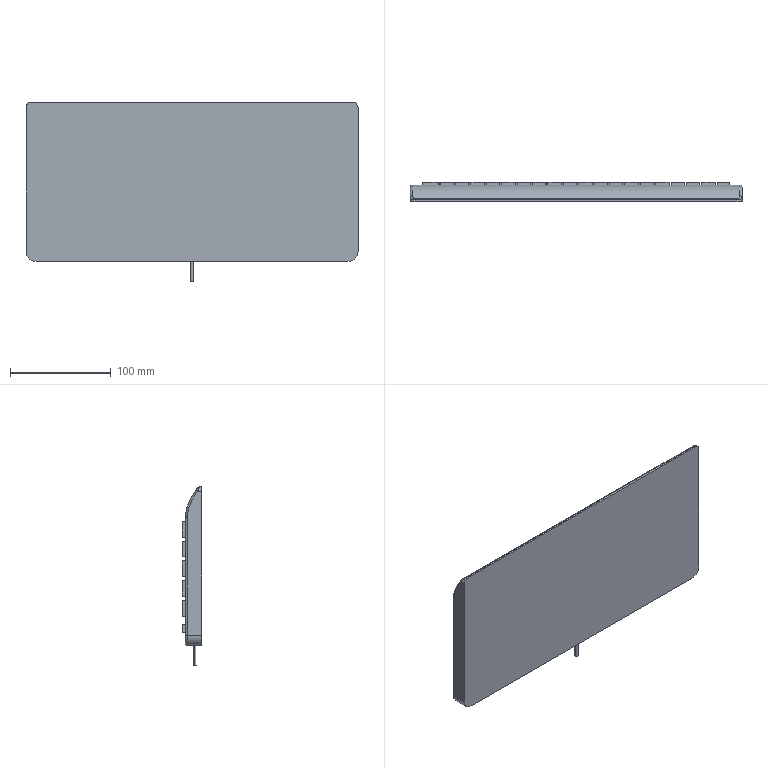Part | SolidWorks | features ICE 7, Fillet 4, LPattern 2, Extrusion 1 | 1 solid | 706 faces | box 330 x 19.5 x 178 mm | volume 879010 mm3 | plane 641 | spline 47 | cylinder 12 | torus 6 | commonest cylinder face diameters 4 x4 20 x3 3 x2 10 x2 94.468 x1